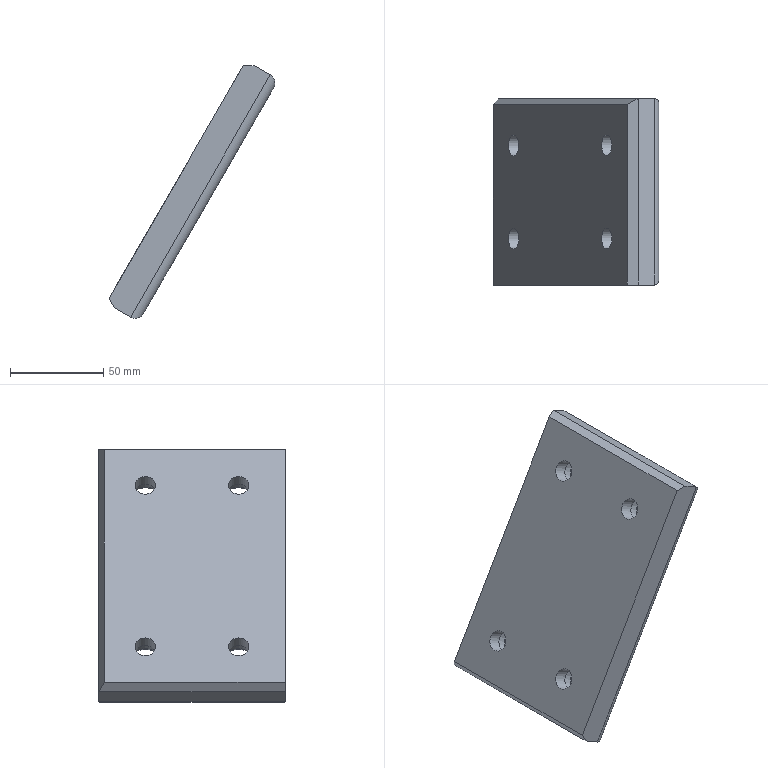Part | NX | features solid 2 | 1 solid | 29 faces | box 88.99 x 100 x 135.574 mm | volume 279727 mm3 | plane 13 | cylinder 12 | torus 4 | commonest cylinder face diameters 10 x4 11 x4 17.5 x4
STEP:
#1=CARTESIAN_POINT('',(245.928,265.,-69.977));
#2=VERTEX_POINT('',#1);
#3=CARTESIAN_POINT('',(241.553,265.,-77.554));
#4=DIRECTION('',(0.866,0.,-0.5));
#5=DIRECTION('',(0.5,0.,0.866));
#6=AXIS2_PLACEMENT_3D('',#3,#4,#5);
#7=CIRCLE('',#6,8.75);
#8=EDGE_CURVE('',#2,#2,#7,.T.);
#9=ORIENTED_EDGE('',*,*,#8,.T.);
#10=EDGE_LOOP('',(#9));
#11=FACE_BOUND('',#10,.T.);
#12=CARTESIAN_POINT('',(229.383,265.,-80.632));
#13=VERTEX_POINT('',#12);
#14=CARTESIAN_POINT('',(233.758,265.,-73.054));
#15=DIRECTION('',(-0.866,0.,0.5));
#16=DIRECTION('',(-0.5,0.,-0.866));
#17=AXIS2_PLACEMENT_3D('',#14,#15,#16);
#18=CIRCLE('',#17,8.75);
#19=EDGE_CURVE('',#13,#13,#18,.T.);
#20=ORIENTED_EDGE('',*,*,#19,.T.);
#21=EDGE_LOOP('',(#20));
#22=FACE_BOUND('',#21,.T.);
#23=CARTESIAN_POINT('',(244.151,265.,-79.054));
#24=DIRECTION('',(-0.866,0.,0.5));
#25=DIRECTION('',(-0.5,0.,-0.866));
#26=AXIS2_PLACEMENT_3D('',#23,#24,#25);
#27=CYLINDRICAL_SURFACE('',#26,8.75);
#28=ADVANCED_FACE('',(#11,#22),#27,.F.);
#29=CARTESIAN_POINT('',(295.928,265.,16.626));
#30=VERTEX_POINT('',#29);
#31=CARTESIAN_POINT('',(291.553,265.,9.048));
#32=DIRECTION('',(0.866,0.,-0.5));
#33=DIRECTION('',(0.5,0.,0.866));
#34=AXIS2_PLACEMENT_3D('',#31,#32,#33);
#35=CIRCLE('',#34,8.75);
#36=EDGE_CURVE('',#30,#30,#35,.T.);
#37=ORIENTED_EDGE('',*,*,#36,.T.);
#38=EDGE_LOOP('',(#37));
#39=FACE_BOUND('',#38,.T.);
#40=CARTESIAN_POINT('',(279.383,265.,5.97));
#41=VERTEX_POINT('',#40);
#42=CARTESIAN_POINT('',(283.758,265.,13.548));
#43=DIRECTION('',(-0.866,0.,0.5));
#44=DIRECTION('',(-0.5,0.,-0.866));
#45=AXIS2_PLACEMENT_3D('',#42,#43,#44);
#46=CIRCLE('',#45,8.75);
#47=EDGE_CURVE('',#41,#41,#46,.T.);
#48=ORIENTED_EDGE('',*,*,#47,.T.);
#49=EDGE_LOOP('',(#48));
#50=FACE_BOUND('',#49,.T.);
#51=CARTESIAN_POINT('',(294.151,265.,7.548));
#52=DIRECTION('',(-0.866,0.,0.5));
#53=DIRECTION('',(-0.5,0.,-0.866));
#54=AXIS2_PLACEMENT_3D('',#51,#52,#53);
#55=CYLINDRICAL_SURFACE('',#54,8.75);
#56=ADVANCED_FACE('',(#39,#50),#55,.F.);
#57=CARTESIAN_POINT('',(231.008,265.,-77.818));
#58=VERTEX_POINT('',#57);
#59=CARTESIAN_POINT('',(233.758,265.,-73.054));
#60=DIRECTION('',(-0.866,0.,0.5));
#61=DIRECTION('',(-0.5,0.,-0.866));
#62=AXIS2_PLACEMENT_3D('',#59,#60,#61);
#63=CIRCLE('',#62,5.5);
#64=EDGE_CURVE('',#58,#58,#63,.T.);
#65=ORIENTED_EDGE('',*,*,#64,.T.);
#66=EDGE_LOOP('',(#65));
#67=FACE_BOUND('',#66,.T.);
#68=ORIENTED_EDGE('',*,*,#19,.F.);
#69=EDGE_LOOP('',(#68));
#70=FACE_BOUND('',#69,.T.);
#71=CARTESIAN_POINT('',(233.758,265.,-73.054));
#72=DIRECTION('',(-0.866,0.,0.5));
#73=DIRECTION('',(-0.5,0.,-0.866));
#74=AXIS2_PLACEMENT_3D('',#71,#72,#73);
#75=PLANE('',#74);
#76=ADVANCED_FACE('',(#67,#70),#75,.F.);
#77=CARTESIAN_POINT('',(281.008,265.,8.785));
#78=VERTEX_POINT('',#77);
#79=CARTESIAN_POINT('',(283.758,265.,13.548));
#80=DIRECTION('',(-0.866,0.,0.5));
#81=DIRECTION('',(-0.5,0.,-0.866));
#82=AXIS2_PLACEMENT_3D('',#79,#80,#81);
#83=CIRCLE('',#82,5.5);
#84=EDGE_CURVE('',#78,#78,#83,.T.);
#85=ORIENTED_EDGE('',*,*,#84,.T.);
#86=EDGE_LOOP('',(#85));
#87=FACE_BOUND('',#86,.T.);
#88=ORIENTED_EDGE('',*,*,#47,.F.);
#89=EDGE_LOOP('',(#88));
#90=FACE_BOUND('',#89,.T.);
#91=CARTESIAN_POINT('',(283.758,265.,13.548));
#92=DIRECTION('',(-0.866,0.,0.5));
#93=DIRECTION('',(-0.5,0.,-0.866));
#94=AXIS2_PLACEMENT_3D('',#91,#92,#93);
#95=PLANE('',#94);
#96=ADVANCED_FACE('',(#87,#90),#95,.F.);
#97=CARTESIAN_POINT('',(227.321,290.,-98.205));
#98=VERTEX_POINT('',#97);
#99=CARTESIAN_POINT('',(218.66,290.,-93.205));
#100=VERTEX_POINT('',#99);
#101=CARTESIAN_POINT('',(231.651,290.,-100.705));
#102=DIRECTION('',(-0.866,0.,0.5));
#103=VECTOR('',#102,1000.);
#104=LINE('',#101,#103);
#105=EDGE_CURVE('',#98,#100,#104,.T.);
#106=ORIENTED_EDGE('',*,*,#105,.T.);
#107=CARTESIAN_POINT('',(293.66,290.,36.699));
#108=VERTEX_POINT('',#107);
#109=CARTESIAN_POINT('',(218.66,290.,-93.205));
#110=DIRECTION('',(0.5,0.,0.866));
#111=VECTOR('',#110,1000.);
#112=LINE('',#109,#111);
#113=EDGE_CURVE('',#100,#108,#112,.T.);
#114=ORIENTED_EDGE('',*,*,#113,.T.);
#115=CARTESIAN_POINT('',(302.321,290.,31.699));
#116=VERTEX_POINT('',#115);
#117=CARTESIAN_POINT('',(293.66,290.,36.699));
#118=CARTESIAN_POINT('',(296.547,290.,35.032));
#119=CARTESIAN_POINT('',(299.434,290.,33.365));
#120=CARTESIAN_POINT('',(302.321,290.,31.699));
#121=B_SPLINE_CURVE_WITH_KNOTS('',3,(#117,#118,#119,#120),.UNSPECIFIED.,.F.,.F.,(4,4),(0.25,0.75),.UNSPECIFIED.);
#122=EDGE_CURVE('',#116,#108,#121,.F.);
#123=ORIENTED_EDGE('',*,*,#122,.F.);
#124=CARTESIAN_POINT('',(227.321,290.,-98.205));
#125=DIRECTION('',(0.5,0.,0.866));
#126=VECTOR('',#125,1000.);
#127=LINE('',#124,#126);
#128=EDGE_CURVE('',#116,#98,#127,.F.);
#129=ORIENTED_EDGE('',*,*,#128,.T.);
#130=EDGE_LOOP('',(#106,#114,#123,#129));
#131=FACE_BOUND('',#130,.T.);
#132=CARTESIAN_POINT('',(231.651,290.,-100.705));
#133=DIRECTION('',(0.,-1.,0.));
#134=DIRECTION('',(-0.1736,0.,-0.9848));
#135=AXIS2_PLACEMENT_3D('',#132,#133,#134);
#136=PLANE('',#135);
#137=ADVANCED_FACE('',(#131),#136,.F.);
#138=ORIENTED_EDGE('',*,*,#8,.F.);
#139=EDGE_LOOP('',(#138));
#140=FACE_BOUND('',#139,.T.);
#141=CARTESIAN_POINT('',(250.026,265.,-68.879));
#142=VERTEX_POINT('',#141);
#143=CARTESIAN_POINT('',(244.151,265.,-79.054));
#144=DIRECTION('',(0.866,0.,-0.5));
#145=DIRECTION('',(0.5,0.,0.866));
#146=AXIS2_PLACEMENT_3D('',#143,#144,#145);
#147=CIRCLE('',#146,11.75);
#148=EDGE_CURVE('',#142,#142,#147,.F.);
#149=ORIENTED_EDGE('',*,*,#148,.F.);
#150=EDGE_LOOP('',(#149));
#151=FACE_BOUND('',#150,.T.);
#152=CARTESIAN_POINT('',(241.553,265.,-77.554));
#153=DIRECTION('',(0.866,0.,-0.5));
#154=DIRECTION('',(0.5,0.,0.866));
#155=AXIS2_PLACEMENT_3D('',#152,#153,#154);
#156=TOROIDAL_SURFACE('',#155,11.75,3.);
#157=ADVANCED_FACE('',(#140,#151),#156,.T.);
#158=ORIENTED_EDGE('',*,*,#36,.F.);
#159=EDGE_LOOP('',(#158));
#160=FACE_BOUND('',#159,.T.);
#161=CARTESIAN_POINT('',(300.026,265.,17.724));
#162=VERTEX_POINT('',#161);
#163=CARTESIAN_POINT('',(294.151,265.,7.548));
#164=DIRECTION('',(0.866,0.,-0.5));
#165=DIRECTION('',(0.5,0.,0.866));
#166=AXIS2_PLACEMENT_3D('',#163,#164,#165);
#167=CIRCLE('',#166,11.75);
#168=EDGE_CURVE('',#162,#162,#167,.F.);
#169=ORIENTED_EDGE('',*,*,#168,.F.);
#170=EDGE_LOOP('',(#169));
#171=FACE_BOUND('',#170,.T.);
#172=CARTESIAN_POINT('',(291.553,265.,9.048));
#173=DIRECTION('',(0.866,0.,-0.5));
#174=DIRECTION('',(0.5,0.,0.866));
#175=AXIS2_PLACEMENT_3D('',#172,#173,#174);
#176=TOROIDAL_SURFACE('',#175,11.75,3.);
#177=ADVANCED_FACE('',(#160,#171),#176,.T.);
#178=ORIENTED_EDGE('',*,*,#64,.F.);
#179=EDGE_LOOP('',(#178));
#180=FACE_BOUND('',#179,.T.);
#181=CARTESIAN_POINT('',(229.58,265.,-64.291));
#182=VERTEX_POINT('',#181);
#183=CARTESIAN_POINT('',(226.83,265.,-69.054));
#184=DIRECTION('',(0.866,0.,-0.5));
#185=DIRECTION('',(0.5,0.,0.866));
#186=AXIS2_PLACEMENT_3D('',#183,#184,#185);
#187=CIRCLE('',#186,5.5);
#188=EDGE_CURVE('',#182,#182,#187,.T.);
#189=ORIENTED_EDGE('',*,*,#188,.F.);
#190=EDGE_LOOP('',(#189));
#191=FACE_BOUND('',#190,.T.);
#192=CARTESIAN_POINT('',(157.548,265.,-29.054));
#193=DIRECTION('',(-0.866,0.,0.5));
#194=DIRECTION('',(-0.5,0.,-0.866));
#195=AXIS2_PLACEMENT_3D('',#192,#193,#194);
#196=CYLINDRICAL_SURFACE('',#195,5.5);
#197=ADVANCED_FACE('',(#180,#191),#196,.F.);
#198=ORIENTED_EDGE('',*,*,#84,.F.);
#199=EDGE_LOOP('',(#198));
#200=FACE_BOUND('',#199,.T.);
#201=CARTESIAN_POINT('',(279.58,265.,22.311));
#202=VERTEX_POINT('',#201);
#203=CARTESIAN_POINT('',(276.83,265.,17.548));
#204=DIRECTION('',(0.866,0.,-0.5));
#205=DIRECTION('',(0.5,0.,0.866));
#206=AXIS2_PLACEMENT_3D('',#203,#204,#205);
#207=CIRCLE('',#206,5.5);
#208=EDGE_CURVE('',#202,#202,#207,.T.);
#209=ORIENTED_EDGE('',*,*,#208,.F.);
#210=EDGE_LOOP('',(#209));
#211=FACE_BOUND('',#210,.T.);
#212=CARTESIAN_POINT('',(207.548,265.,57.548));
#213=DIRECTION('',(-0.866,0.,0.5));
#214=DIRECTION('',(-0.5,0.,-0.866));
#215=AXIS2_PLACEMENT_3D('',#212,#213,#214);
#216=CYLINDRICAL_SURFACE('',#215,5.5);
#217=ADVANCED_FACE('',(#200,#211),#216,.F.);
#218=CARTESIAN_POINT('',(304.151,285.,24.869));
#219=VERTEX_POINT('',#218);
#220=CARTESIAN_POINT('',(299.821,285.,27.369));
#221=DIRECTION('',(-0.3536,0.7071,-0.6124));
#222=DIRECTION('',(0.3536,0.7071,0.6124));
#223=AXIS2_PLACEMENT_3D('',#220,#221,#222);
#224=ELLIPSE('',#223,7.071,5.);
#225=EDGE_CURVE('',#116,#219,#224,.T.);
#226=ORIENTED_EDGE('',*,*,#225,.T.);
#227=CARTESIAN_POINT('',(234.151,285.,-96.375));
#228=VERTEX_POINT('',#227);
#229=CARTESIAN_POINT('',(306.651,285.,29.199));
#230=DIRECTION('',(0.5,0.,0.866));
#231=VECTOR('',#230,1000.);
#232=LINE('',#229,#231);
#233=EDGE_CURVE('',#228,#219,#232,.T.);
#234=ORIENTED_EDGE('',*,*,#233,.F.);
#235=CARTESIAN_POINT('',(229.821,285.,-93.875));
#236=DIRECTION('',(-0.3536,-0.7071,-0.6124));
#237=DIRECTION('',(-0.3536,0.7071,-0.6124));
#238=AXIS2_PLACEMENT_3D('',#235,#236,#237);
#239=ELLIPSE('',#238,7.071,5.);
#240=EDGE_CURVE('',#98,#228,#239,.T.);
#241=ORIENTED_EDGE('',*,*,#240,.F.);
#242=ORIENTED_EDGE('',*,*,#128,.F.);
#243=EDGE_LOOP('',(#226,#234,#241,#242));
#244=FACE_BOUND('',#243,.T.);
#245=CARTESIAN_POINT('',(227.321,285.,-98.205));
#246=DIRECTION('',(-0.5,0.,-0.866));
#247=DIRECTION('',(0.866,0.,-0.5));
#248=AXIS2_PLACEMENT_3D('',#245,#246,#247);
#249=CYLINDRICAL_SURFACE('',#248,5.);
#250=ADVANCED_FACE('',(#244),#249,.T.);
#251=CARTESIAN_POINT('',(215.83,287.,-88.107));
#252=VERTEX_POINT('',#251);
#253=CARTESIAN_POINT('',(216.422,287.628,-89.174));
#254=DIRECTION('',(-0.4316,-0.4575,0.7774));
#255=VECTOR('',#254,1000.);
#256=LINE('',#253,#255);
#257=EDGE_CURVE('',#100,#252,#256,.T.);
#258=ORIENTED_EDGE('',*,*,#257,.T.);
#259=CARTESIAN_POINT('',(287.83,287.,36.601));
#260=VERTEX_POINT('',#259);
#261=CARTESIAN_POINT('',(214.33,287.,-90.705));
#262=DIRECTION('',(-0.5,0.,-0.866));
#263=VECTOR('',#262,1000.);
#264=LINE('',#261,#263);
#265=EDGE_CURVE('',#260,#252,#264,.T.);
#266=ORIENTED_EDGE('',*,*,#265,.F.);
#267=CARTESIAN_POINT('',(293.66,290.,36.699));
#268=DIRECTION('',(-0.8891,-0.4575,-0.01496));
#269=VECTOR('',#268,1000.);
#270=LINE('',#267,#269);
#271=EDGE_CURVE('',#260,#108,#270,.F.);
#272=ORIENTED_EDGE('',*,*,#271,.T.);
#273=ORIENTED_EDGE('',*,*,#113,.F.);
#274=EDGE_LOOP('',(#258,#266,#272,#273));
#275=FACE_BOUND('',#274,.T.);
#276=CARTESIAN_POINT('',(218.66,290.,-93.205));
#277=DIRECTION('',(0.4456,-0.8575,-0.2572));
#278=DIRECTION('',(0.8579,0.4911,-0.1513));
#279=AXIS2_PLACEMENT_3D('',#276,#277,#278);
#280=PLANE('',#279);
#281=ADVANCED_FACE('',(#275),#280,.F.);
#282=CARTESIAN_POINT('',(218.66,190.,-93.205));
#283=VERTEX_POINT('',#282);
#284=CARTESIAN_POINT('',(215.83,190.,-88.107));
#285=VERTEX_POINT('',#284);
#286=CARTESIAN_POINT('',(215.83,190.,-88.107));
#287=DIRECTION('',(-0.4854,0.,0.8743));
#288=VECTOR('',#287,1000.);
#289=LINE('',#286,#288);
#290=EDGE_CURVE('',#283,#285,#289,.T.);
#291=ORIENTED_EDGE('',*,*,#290,.T.);
#292=CARTESIAN_POINT('',(215.83,140.,-88.107));
#293=DIRECTION('',(0.,-1.,0.));
#294=VECTOR('',#293,1000.);
#295=LINE('',#292,#294);
#296=EDGE_CURVE('',#252,#285,#295,.T.);
#297=ORIENTED_EDGE('',*,*,#296,.F.);
#298=ORIENTED_EDGE('',*,*,#257,.F.);
#299=CARTESIAN_POINT('',(218.66,290.,-93.205));
#300=DIRECTION('',(0.,1.,0.));
#301=VECTOR('',#300,1000.);
#302=LINE('',#299,#301);
#303=EDGE_CURVE('',#283,#100,#302,.T.);
#304=ORIENTED_EDGE('',*,*,#303,.F.);
#305=EDGE_LOOP('',(#291,#297,#298,#304));
#306=FACE_BOUND('',#305,.T.);
#307=CARTESIAN_POINT('',(215.83,290.,-88.107));
#308=DIRECTION('',(-0.8743,0.,-0.4854));
#309=DIRECTION('',(0.4854,0.,-0.8743));
#310=AXIS2_PLACEMENT_3D('',#307,#308,#309);
#311=PLANE('',#310);
#312=ADVANCED_FACE('',(#306),#311,.T.);
#313=CARTESIAN_POINT('',(287.83,190.,36.601));
#314=VERTEX_POINT('',#313);
#315=CARTESIAN_POINT('',(287.83,290.,36.601));
#316=DIRECTION('',(0.,1.,0.));
#317=VECTOR('',#316,1000.);
#318=LINE('',#315,#317);
#319=EDGE_CURVE('',#314,#260,#318,.T.);
#320=ORIENTED_EDGE('',*,*,#319,.F.);
#321=CARTESIAN_POINT('',(293.66,190.,36.699));
#322=VERTEX_POINT('',#321);
#323=CARTESIAN_POINT('',(229.357,190.,35.617));
#324=DIRECTION('',(0.9999,0.,0.01682));
#325=VECTOR('',#324,1000.);
#326=LINE('',#323,#325);
#327=EDGE_CURVE('',#322,#314,#326,.F.);
#328=ORIENTED_EDGE('',*,*,#327,.F.);
#329=CARTESIAN_POINT('',(293.66,290.,36.699));
#330=DIRECTION('',(0.,-1.,0.));
#331=VECTOR('',#330,1000.);
#332=LINE('',#329,#331);
#333=EDGE_CURVE('',#108,#322,#332,.T.);
#334=ORIENTED_EDGE('',*,*,#333,.F.);
#335=ORIENTED_EDGE('',*,*,#271,.F.);
#336=EDGE_LOOP('',(#320,#328,#334,#335));
#337=FACE_BOUND('',#336,.T.);
#338=CARTESIAN_POINT('',(293.66,290.,36.699));
#339=DIRECTION('',(0.01682,0.,-0.9999));
#340=DIRECTION('',(0.9999,0.,0.01682));
#341=AXIS2_PLACEMENT_3D('',#338,#339,#340);
#342=PLANE('',#341);
#343=ADVANCED_FACE('',(#337),#342,.F.);
#344=ORIENTED_EDGE('',*,*,#296,.T.);
#345=CARTESIAN_POINT('',(214.33,190.,-90.705));
#346=DIRECTION('',(0.5,0.,0.866));
#347=VECTOR('',#346,1000.);
#348=LINE('',#345,#347);
#349=EDGE_CURVE('',#285,#314,#348,.T.);
#350=ORIENTED_EDGE('',*,*,#349,.T.);
#351=ORIENTED_EDGE('',*,*,#319,.T.);
#352=ORIENTED_EDGE('',*,*,#265,.T.);
#353=EDGE_LOOP('',(#344,#350,#351,#352));
#354=FACE_BOUND('',#353,.T.);
#355=ORIENTED_EDGE('',*,*,#188,.T.);
#356=EDGE_LOOP('',(#355));
#357=FACE_BOUND('',#356,.T.);
#358=ORIENTED_EDGE('',*,*,#208,.T.);
#359=EDGE_LOOP('',(#358));
#360=FACE_BOUND('',#359,.T.);
#361=CARTESIAN_POINT('',(229.58,215.,-64.291));
#362=VERTEX_POINT('',#361);
#363=CARTESIAN_POINT('',(226.83,215.,-69.054));
#364=DIRECTION('',(0.866,0.,-0.5));
#365=DIRECTION('',(0.5,0.,0.866));
#366=AXIS2_PLACEMENT_3D('',#363,#364,#365);
#367=CIRCLE('',#366,5.5);
#368=EDGE_CURVE('',#362,#362,#367,.T.);
#369=ORIENTED_EDGE('',*,*,#368,.T.);
#370=EDGE_LOOP('',(#369));
#371=FACE_BOUND('',#370,.T.);
#372=CARTESIAN_POINT('',(279.58,215.,22.311));
#373=VERTEX_POINT('',#372);
#374=CARTESIAN_POINT('',(276.83,215.,17.548));
#375=DIRECTION('',(0.866,0.,-0.5));
#376=DIRECTION('',(0.5,0.,0.866));
#377=AXIS2_PLACEMENT_3D('',#374,#375,#376);
#378=CIRCLE('',#377,5.5);
#379=EDGE_CURVE('',#373,#373,#378,.T.);
#380=ORIENTED_EDGE('',*,*,#379,.T.);
#381=EDGE_LOOP('',(#380));
#382=FACE_BOUND('',#381,.T.);
#383=CARTESIAN_POINT('',(214.33,290.,-90.705));
#384=DIRECTION('',(0.866,0.,-0.5));
#385=DIRECTION('',(0.5,0.,0.866));
#386=AXIS2_PLACEMENT_3D('',#383,#384,#385);
#387=PLANE('',#386);
#388=ADVANCED_FACE('',(#354,#357,#360,#371,#382),#387,.F.);
#389=CARTESIAN_POINT('',(234.151,195.,-96.375));
#390=VERTEX_POINT('',#389);
#391=CARTESIAN_POINT('',(227.321,190.,-98.205));
#392=VERTEX_POINT('',#391);
#393=CARTESIAN_POINT('',(229.821,195.,-93.875));
#394=DIRECTION('',(0.3536,-0.7071,0.6124));
#395=DIRECTION('',(0.3536,0.7071,0.6124));
#396=AXIS2_PLACEMENT_3D('',#393,#394,#395);
#397=ELLIPSE('',#396,7.071,5.);
#398=EDGE_CURVE('',#390,#392,#397,.F.);
#399=ORIENTED_EDGE('',*,*,#398,.T.);
#400=CARTESIAN_POINT('',(227.321,290.,-98.205));
#401=DIRECTION('',(0.,-1.,0.));
#402=VECTOR('',#401,1000.);
#403=LINE('',#400,#402);
#404=EDGE_CURVE('',#98,#392,#403,.T.);
#405=ORIENTED_EDGE('',*,*,#404,.F.);
#406=ORIENTED_EDGE('',*,*,#240,.T.);
#407=CARTESIAN_POINT('',(234.151,290.,-96.375));
#408=DIRECTION('',(0.,-1.,0.));
#409=VECTOR('',#408,1000.);
#410=LINE('',#407,#409);
#411=EDGE_CURVE('',#390,#228,#410,.F.);
#412=ORIENTED_EDGE('',*,*,#411,.F.);
#413=EDGE_LOOP('',(#399,#405,#406,#412));
#414=FACE_BOUND('',#413,.T.);
#415=CARTESIAN_POINT('',(229.821,290.,-93.875));
#416=DIRECTION('',(0.,-1.,0.));
#417=DIRECTION('',(-0.1736,0.,-0.9848));
#418=AXIS2_PLACEMENT_3D('',#415,#416,#417);
#419=CYLINDRICAL_SURFACE('',#418,5.);
#420=ADVANCED_FACE('',(#414),#419,.T.);
#421=CARTESIAN_POINT('',(304.151,195.,24.869));
#422=VERTEX_POINT('',#421);
#423=CARTESIAN_POINT('',(302.321,190.,31.699));
#424=VERTEX_POINT('',#423);
#425=CARTESIAN_POINT('',(299.821,195.,27.369));
#426=DIRECTION('',(0.3536,0.7071,0.6124));
#427=DIRECTION('',(0.3536,-0.7071,0.6124));
#428=AXIS2_PLACEMENT_3D('',#425,#426,#427);
#429=ELLIPSE('',#428,7.071,5.);
#430=EDGE_CURVE('',#422,#424,#429,.F.);
#431=ORIENTED_EDGE('',*,*,#430,.F.);
#432=CARTESIAN_POINT('',(304.151,140.,24.869));
#433=DIRECTION('',(0.,-1.,0.));
#434=VECTOR('',#433,1000.);
#435=LINE('',#432,#434);
#436=EDGE_CURVE('',#219,#422,#435,.T.);
#437=ORIENTED_EDGE('',*,*,#436,.F.);
#438=ORIENTED_EDGE('',*,*,#225,.F.);
#439=CARTESIAN_POINT('',(302.321,290.,31.699));
#440=DIRECTION('',(0.,-1.,0.));
#441=VECTOR('',#440,1000.);
#442=LINE('',#439,#441);
#443=EDGE_CURVE('',#424,#116,#442,.F.);
#444=ORIENTED_EDGE('',*,*,#443,.F.);
#445=EDGE_LOOP('',(#431,#437,#438,#444));
#446=FACE_BOUND('',#445,.T.);
#447=CARTESIAN_POINT('',(299.821,290.,27.369));
#448=DIRECTION('',(0.,1.,0.));
#449=DIRECTION('',(0.1736,0.,0.9848));
#450=AXIS2_PLACEMENT_3D('',#447,#448,#449);
#451=CYLINDRICAL_SURFACE('',#450,5.);
#452=ADVANCED_FACE('',(#446),#451,.T.);
#453=ORIENTED_EDGE('',*,*,#411,.T.);
#454=ORIENTED_EDGE('',*,*,#233,.T.);
#455=ORIENTED_EDGE('',*,*,#436,.T.);
#456=CARTESIAN_POINT('',(231.651,195.,-100.705));
#457=DIRECTION('',(0.5,0.,0.866));
#458=VECTOR('',#457,1000.);
#459=LINE('',#456,#458);
#460=EDGE_CURVE('',#422,#390,#459,.F.);
#461=ORIENTED_EDGE('',*,*,#460,.T.);
#462=EDGE_LOOP('',(#453,#454,#455,#461));
#463=FACE_BOUND('',#462,.T.);
#464=ORIENTED_EDGE('',*,*,#148,.T.);
#465=EDGE_LOOP('',(#464));
#466=FACE_BOUND('',#465,.T.);
#467=ORIENTED_EDGE('',*,*,#168,.T.);
#468=EDGE_LOOP('',(#467));
#469=FACE_BOUND('',#468,.T.);
#470=CARTESIAN_POINT('',(250.026,215.,-68.879));
#471=VERTEX_POINT('',#470);
#472=CARTESIAN_POINT('',(244.151,215.,-79.054));
#473=DIRECTION('',(0.866,0.,-0.5));
#474=DIRECTION('',(0.5,0.,0.866));
#475=AXIS2_PLACEMENT_3D('',#472,#473,#474);
#476=CIRCLE('',#475,11.75);
#477=EDGE_CURVE('',#471,#471,#476,.F.);
#478=ORIENTED_EDGE('',*,*,#477,.T.);
#479=EDGE_LOOP('',(#478));
#480=FACE_BOUND('',#479,.T.);
#481=CARTESIAN_POINT('',(300.026,215.,17.724));
#482=VERTEX_POINT('',#481);
#483=CARTESIAN_POINT('',(294.151,215.,7.548));
#484=DIRECTION('',(0.866,0.,-0.5));
#485=DIRECTION('',(0.5,0.,0.866));
#486=AXIS2_PLACEMENT_3D('',#483,#484,#485);
#487=CIRCLE('',#486,11.75);
#488=EDGE_CURVE('',#482,#482,#487,.F.);
#489=ORIENTED_EDGE('',*,*,#488,.T.);
#490=EDGE_LOOP('',(#489));
#491=FACE_BOUND('',#490,.T.);
#492=CARTESIAN_POINT('',(231.651,290.,-100.705));
#493=DIRECTION('',(0.866,0.,-0.5));
#494=DIRECTION('',(0.5,0.,0.866));
#495=AXIS2_PLACEMENT_3D('',#492,#493,#494);
#496=PLANE('',#495);
#497=ADVANCED_FACE('',(#463,#466,#469,#480,#491),#496,.T.);
#498=ORIENTED_EDGE('',*,*,#443,.T.);
#499=ORIENTED_EDGE('',*,*,#122,.T.);
#500=ORIENTED_EDGE('',*,*,#333,.T.);
#501=CARTESIAN_POINT('',(293.66,190.,36.699));
#502=CARTESIAN_POINT('',(296.547,190.,35.032));
#503=CARTESIAN_POINT('',(299.434,190.,33.365));
#504=CARTESIAN_POINT('',(302.321,190.,31.699));
#505=B_SPLINE_CURVE_WITH_KNOTS('',3,(#501,#502,#503,#504),.UNSPECIFIED.,.F.,.F.,(4,4),(0.,1.),.UNSPECIFIED.);
#506=EDGE_CURVE('',#424,#322,#505,.F.);
#507=ORIENTED_EDGE('',*,*,#506,.F.);
#508=EDGE_LOOP('',(#498,#499,#500,#507));
#509=FACE_BOUND('',#508,.T.);
#510=CARTESIAN_POINT('',(306.651,290.,29.199));
#511=DIRECTION('',(-0.5,0.,-0.866));
#512=DIRECTION('',(0.866,0.,-0.5));
#513=AXIS2_PLACEMENT_3D('',#510,#511,#512);
#514=PLANE('',#513);
#515=ADVANCED_FACE('',(#509),#514,.F.);
#516=ORIENTED_EDGE('',*,*,#303,.T.);
#517=ORIENTED_EDGE('',*,*,#105,.F.);
#518=ORIENTED_EDGE('',*,*,#404,.T.);
#519=CARTESIAN_POINT('',(231.651,190.,-100.705));
#520=DIRECTION('',(-0.866,0.,0.5));
#521=VECTOR('',#520,1000.);
#522=LINE('',#519,#521);
#523=EDGE_CURVE('',#392,#283,#522,.T.);
#524=ORIENTED_EDGE('',*,*,#523,.T.);
#525=EDGE_LOOP('',(#516,#517,#518,#524));
#526=FACE_BOUND('',#525,.T.);
#527=CARTESIAN_POINT('',(231.651,290.,-100.705));
#528=DIRECTION('',(-0.5,0.,-0.866));
#529=DIRECTION('',(0.866,0.,-0.5));
#530=AXIS2_PLACEMENT_3D('',#527,#528,#529);
#531=PLANE('',#530);
#532=ADVANCED_FACE('',(#526),#531,.T.);
#533=ORIENTED_EDGE('',*,*,#349,.F.);
#534=ORIENTED_EDGE('',*,*,#290,.F.);
#535=ORIENTED_EDGE('',*,*,#523,.F.);
#536=CARTESIAN_POINT('',(227.321,190.,-98.205));
#537=DIRECTION('',(0.5,0.,0.866));
#538=VECTOR('',#537,1000.);
#539=LINE('',#536,#538);
#540=EDGE_CURVE('',#392,#424,#539,.T.);
#541=ORIENTED_EDGE('',*,*,#540,.T.);
#542=ORIENTED_EDGE('',*,*,#506,.T.);
#543=ORIENTED_EDGE('',*,*,#327,.T.);
#544=EDGE_LOOP('',(#533,#534,#535,#541,#542,#543));
#545=FACE_BOUND('',#544,.T.);
#546=CARTESIAN_POINT('',(231.651,190.,-100.705));
#547=DIRECTION('',(0.,-1.,0.));
#548=DIRECTION('',(-0.1736,0.,-0.9848));
#549=AXIS2_PLACEMENT_3D('',#546,#547,#548);
#550=PLANE('',#549);
#551=ADVANCED_FACE('',(#545),#550,.T.);
#552=CARTESIAN_POINT('',(281.008,215.,8.785));
#553=VERTEX_POINT('',#552);
#554=CARTESIAN_POINT('',(283.758,215.,13.548));
#555=DIRECTION('',(-0.866,0.,0.5));
#556=DIRECTION('',(-0.5,0.,-0.866));
#557=AXIS2_PLACEMENT_3D('',#554,#555,#556);
#558=CIRCLE('',#557,5.5);
#559=EDGE_CURVE('',#553,#553,#558,.T.);
#560=ORIENTED_EDGE('',*,*,#559,.F.);
#561=EDGE_LOOP('',(#560));
#562=FACE_BOUND('',#561,.T.);
#563=ORIENTED_EDGE('',*,*,#379,.F.);
#564=EDGE_LOOP('',(#563));
#565=FACE_BOUND('',#564,.T.);
#566=CARTESIAN_POINT('',(207.548,215.,57.548));
#567=DIRECTION('',(-0.866,0.,0.5));
#568=DIRECTION('',(-0.5,0.,-0.866));
#569=AXIS2_PLACEMENT_3D('',#566,#567,#568);
#570=CYLINDRICAL_SURFACE('',#569,5.5);
#571=ADVANCED_FACE('',(#562,#565),#570,.F.);
#572=ORIENTED_EDGE('',*,*,#559,.T.);
#573=EDGE_LOOP('',(#572));
#574=FACE_BOUND('',#573,.T.);
#575=CARTESIAN_POINT('',(279.383,215.,5.97));
#576=VERTEX_POINT('',#575);
#577=CARTESIAN_POINT('',(283.758,215.,13.548));
#578=DIRECTION('',(-0.866,0.,0.5));
#579=DIRECTION('',(-0.5,0.,-0.866));
#580=AXIS2_PLACEMENT_3D('',#577,#578,#579);
#581=CIRCLE('',#580,8.75);
#582=EDGE_CURVE('',#576,#576,#581,.T.);
#583=ORIENTED_EDGE('',*,*,#582,.F.);
#584=EDGE_LOOP('',(#583));
#585=FACE_BOUND('',#584,.T.);
#586=CARTESIAN_POINT('',(283.758,215.,13.548));
#587=DIRECTION('',(-0.866,0.,0.5));
#588=DIRECTION('',(-0.5,0.,-0.866));
#589=AXIS2_PLACEMENT_3D('',#586,#587,#588);
#590=PLANE('',#589);
#591=ADVANCED_FACE('',(#574,#585),#590,.F.);
#592=CARTESIAN_POINT('',(295.928,215.,16.626));
#593=VERTEX_POINT('',#592);
#594=CARTESIAN_POINT('',(291.553,215.,9.048));
#595=DIRECTION('',(0.866,0.,-0.5));
#596=DIRECTION('',(0.5,0.,0.866));
#597=AXIS2_PLACEMENT_3D('',#594,#595,#596);
#598=CIRCLE('',#597,8.75);
#599=EDGE_CURVE('',#593,#593,#598,.T.);
#600=ORIENTED_EDGE('',*,*,#599,.T.);
#601=EDGE_LOOP('',(#600));
#602=FACE_BOUND('',#601,.T.);
#603=ORIENTED_EDGE('',*,*,#582,.T.);
#604=EDGE_LOOP('',(#603));
#605=FACE_BOUND('',#604,.T.);
#606=CARTESIAN_POINT('',(294.151,215.,7.548));
#607=DIRECTION('',(-0.866,0.,0.5));
#608=DIRECTION('',(-0.5,0.,-0.866));
#609=AXIS2_PLACEMENT_3D('',#606,#607,#608);
#610=CYLINDRICAL_SURFACE('',#609,8.75);
#611=ADVANCED_FACE('',(#602,#605),#610,.F.);
#612=CARTESIAN_POINT('',(231.008,215.,-77.818));
#613=VERTEX_POINT('',#612);
#614=CARTESIAN_POINT('',(233.758,215.,-73.054));
#615=DIRECTION('',(-0.866,0.,0.5));
#616=DIRECTION('',(-0.5,0.,-0.866));
#617=AXIS2_PLACEMENT_3D('',#614,#615,#616);
#618=CIRCLE('',#617,5.5);
#619=EDGE_CURVE('',#613,#613,#618,.T.);
#620=ORIENTED_EDGE('',*,*,#619,.F.);
#621=EDGE_LOOP('',(#620));
#622=FACE_BOUND('',#621,.T.);
#623=ORIENTED_EDGE('',*,*,#368,.F.);
#624=EDGE_LOOP('',(#623));
#625=FACE_BOUND('',#624,.T.);
#626=CARTESIAN_POINT('',(157.548,215.,-29.054));
#627=DIRECTION('',(-0.866,0.,0.5));
#628=DIRECTION('',(-0.5,0.,-0.866));
#629=AXIS2_PLACEMENT_3D('',#626,#627,#628);
#630=CYLINDRICAL_SURFACE('',#629,5.5);
#631=ADVANCED_FACE('',(#622,#625),#630,.F.);
#632=ORIENTED_EDGE('',*,*,#619,.T.);
#633=EDGE_LOOP('',(#632));
#634=FACE_BOUND('',#633,.T.);
#635=CARTESIAN_POINT('',(229.383,215.,-80.632));
#636=VERTEX_POINT('',#635);
#637=CARTESIAN_POINT('',(233.758,215.,-73.054));
#638=DIRECTION('',(-0.866,0.,0.5));
#639=DIRECTION('',(-0.5,0.,-0.866));
#640=AXIS2_PLACEMENT_3D('',#637,#638,#639);
#641=CIRCLE('',#640,8.75);
#642=EDGE_CURVE('',#636,#636,#641,.T.);
#643=ORIENTED_EDGE('',*,*,#642,.F.);
#644=EDGE_LOOP('',(#643));
#645=FACE_BOUND('',#644,.T.);
#646=CARTESIAN_POINT('',(233.758,215.,-73.054));
#647=DIRECTION('',(-0.866,0.,0.5));
#648=DIRECTION('',(-0.5,0.,-0.866));
#649=AXIS2_PLACEMENT_3D('',#646,#647,#648);
#650=PLANE('',#649);
#651=ADVANCED_FACE('',(#634,#645),#650,.F.);
#652=CARTESIAN_POINT('',(245.928,215.,-69.977));
#653=VERTEX_POINT('',#652);
#654=CARTESIAN_POINT('',(241.553,215.,-77.554));
#655=DIRECTION('',(0.866,0.,-0.5));
#656=DIRECTION('',(0.5,0.,0.866));
#657=AXIS2_PLACEMENT_3D('',#654,#655,#656);
#658=CIRCLE('',#657,8.75);
#659=EDGE_CURVE('',#653,#653,#658,.T.);
#660=ORIENTED_EDGE('',*,*,#659,.T.);
#661=EDGE_LOOP('',(#660));
#662=FACE_BOUND('',#661,.T.);
#663=ORIENTED_EDGE('',*,*,#642,.T.);
#664=EDGE_LOOP('',(#663));
#665=FACE_BOUND('',#664,.T.);
#666=CARTESIAN_POINT('',(244.151,215.,-79.054));
#667=DIRECTION('',(-0.866,0.,0.5));
#668=DIRECTION('',(-0.5,0.,-0.866));
#669=AXIS2_PLACEMENT_3D('',#666,#667,#668);
#670=CYLINDRICAL_SURFACE('',#669,8.75);
#671=ADVANCED_FACE('',(#662,#665),#670,.F.);
#672=ORIENTED_EDGE('',*,*,#430,.T.);
#673=ORIENTED_EDGE('',*,*,#540,.F.);
#674=ORIENTED_EDGE('',*,*,#398,.F.);
#675=ORIENTED_EDGE('',*,*,#460,.F.);
#676=EDGE_LOOP('',(#672,#673,#674,#675));
#677=FACE_BOUND('',#676,.T.);
#678=CARTESIAN_POINT('',(227.321,195.,-98.205));
#679=DIRECTION('',(0.5,0.,0.866));
#680=DIRECTION('',(-0.866,0.,0.5));
#681=AXIS2_PLACEMENT_3D('',#678,#679,#680);
#682=CYLINDRICAL_SURFACE('',#681,5.);
#683=ADVANCED_FACE('',(#677),#682,.T.);
#684=ORIENTED_EDGE('',*,*,#659,.F.);
#685=EDGE_LOOP('',(#684));
#686=FACE_BOUND('',#685,.T.);
#687=ORIENTED_EDGE('',*,*,#477,.F.);
#688=EDGE_LOOP('',(#687));
#689=FACE_BOUND('',#688,.T.);
#690=CARTESIAN_POINT('',(241.553,215.,-77.554));
#691=DIRECTION('',(0.866,0.,-0.5));
#692=DIRECTION('',(0.5,0.,0.866));
#693=AXIS2_PLACEMENT_3D('',#690,#691,#692);
#694=TOROIDAL_SURFACE('',#693,11.75,3.);
#695=ADVANCED_FACE('',(#686,#689),#694,.T.);
#696=ORIENTED_EDGE('',*,*,#599,.F.);
#697=EDGE_LOOP('',(#696));
#698=FACE_BOUND('',#697,.T.);
#699=ORIENTED_EDGE('',*,*,#488,.F.);
#700=EDGE_LOOP('',(#699));
#701=FACE_BOUND('',#700,.T.);
#702=CARTESIAN_POINT('',(291.553,215.,9.048));
#703=DIRECTION('',(0.866,0.,-0.5));
#704=DIRECTION('',(0.5,0.,0.866));
#705=AXIS2_PLACEMENT_3D('',#702,#703,#704);
#706=TOROIDAL_SURFACE('',#705,11.75,3.);
#707=ADVANCED_FACE('',(#698,#701),#706,.T.);
#708=CLOSED_SHELL('',(#28,#56,#76,#96,#137,#157,#177,#197,#217,#250,#281,#312,#343,#388,#420,#452,#497,#515,#532,#551,#571,#591,#611,#631,#651,#671,#683,#695,#707));
#709=MANIFOLD_SOLID_BREP('',#708);
#710=(LENGTH_UNIT()NAMED_UNIT(*)SI_UNIT(.MILLI.,.METRE.));
#711=UNCERTAINTY_MEASURE_WITH_UNIT(LENGTH_MEASURE(0.0508),#710,'','');
#712=(NAMED_UNIT(*)PLANE_ANGLE_UNIT()SI_UNIT($,.RADIAN.));
#713=(NAMED_UNIT(*)SI_UNIT($,.STERADIAN.)SOLID_ANGLE_UNIT());
#714=(GEOMETRIC_REPRESENTATION_CONTEXT(3)GLOBAL_UNCERTAINTY_ASSIGNED_CONTEXT((#711))GLOBAL_UNIT_ASSIGNED_CONTEXT((#710,#712,#713))REPRESENTATION_CONTEXT('',''));
#715=ADVANCED_BREP_SHAPE_REPRESENTATION('',(#709),#714);